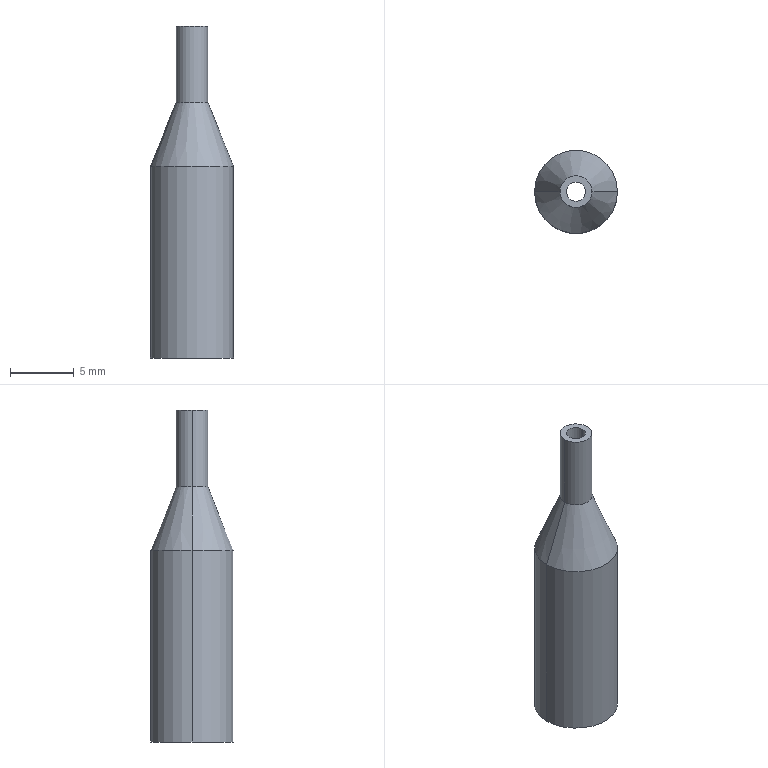Part | SolidWorks | features ICE 2, Chamfer 1, Extrusion 1, HoleWzd 1 | 1 solid | 14 faces | box 6.5 x 6.5 x 26 mm | volume 380.573 mm3 | cylinder 8 | cone 4 | plane 2 | commonest cylinder face diameters 1.5 x2 2.5 x2 4.2 x2 6.5 x2
STEP:
#1=CARTESIAN_POINT('',(-0.75,0.,15.811));
#2=VERTEX_POINT('',#1);
#3=CARTESIAN_POINT('',(0.75,0.,15.811));
#4=VERTEX_POINT('',#3);
#5=CARTESIAN_POINT('',(0.,0.,15.811));
#6=DIRECTION('',(0.,0.,1.));
#7=DIRECTION('',(-1.,0.,0.));
#8=AXIS2_PLACEMENT_3D('',#5,#6,#7);
#9=CIRCLE('',#8,0.75);
#10=EDGE_CURVE('',#2,#4,#9,.T.);
#11=ORIENTED_EDGE('',*,*,#10,.F.);
#12=CARTESIAN_POINT('',(-0.75,0.,26.));
#13=VERTEX_POINT('',#12);
#14=CARTESIAN_POINT('',(-0.75,0.,0.));
#15=DIRECTION('',(0.,0.,1.));
#16=VECTOR('',#15,1000.);
#17=LINE('',#14,#16);
#18=EDGE_CURVE('',#2,#13,#17,.T.);
#19=ORIENTED_EDGE('',*,*,#18,.T.);
#20=CARTESIAN_POINT('',(0.75,0.,26.));
#21=VERTEX_POINT('',#20);
#22=CARTESIAN_POINT('',(0.,0.,26.));
#23=DIRECTION('',(0.,0.,1.));
#24=DIRECTION('',(1.,0.,0.));
#25=AXIS2_PLACEMENT_3D('',#22,#23,#24);
#26=CIRCLE('',#25,0.75);
#27=EDGE_CURVE('',#13,#21,#26,.T.);
#28=ORIENTED_EDGE('',*,*,#27,.T.);
#29=CARTESIAN_POINT('',(0.75,0.,0.));
#30=DIRECTION('',(0.,0.,1.));
#31=VECTOR('',#30,1000.);
#32=LINE('',#29,#31);
#33=EDGE_CURVE('',#4,#21,#32,.T.);
#34=ORIENTED_EDGE('',*,*,#33,.F.);
#35=EDGE_LOOP('',(#11,#19,#28,#34));
#36=FACE_OUTER_BOUND('',#35,.T.);
#37=CARTESIAN_POINT('',(0.,0.,0.));
#38=DIRECTION('',(0.,0.,1.));
#39=DIRECTION('',(1.,0.,0.));
#40=AXIS2_PLACEMENT_3D('',#37,#38,#39);
#41=CYLINDRICAL_SURFACE('',#40,0.75);
#42=ADVANCED_FACE('',(#36),#41,.F.);
#43=CARTESIAN_POINT('',(2.1,0.,15.));
#44=VERTEX_POINT('',#43);
#45=CARTESIAN_POINT('',(-2.1,0.,15.));
#46=VERTEX_POINT('',#45);
#47=CARTESIAN_POINT('',(0.,0.,15.));
#48=DIRECTION('',(0.,0.,-1.));
#49=DIRECTION('',(-1.,0.,0.));
#50=AXIS2_PLACEMENT_3D('',#47,#48,#49);
#51=CIRCLE('',#50,2.1);
#52=EDGE_CURVE('',#44,#46,#51,.T.);
#53=ORIENTED_EDGE('',*,*,#52,.F.);
#54=CARTESIAN_POINT('',(2.1,0.,0.));
#55=VERTEX_POINT('',#54);
#56=CARTESIAN_POINT('',(2.1,0.,0.));
#57=DIRECTION('',(0.,0.,-1.));
#58=VECTOR('',#57,1000.);
#59=LINE('',#56,#58);
#60=EDGE_CURVE('',#44,#55,#59,.T.);
#61=ORIENTED_EDGE('',*,*,#60,.T.);
#62=CARTESIAN_POINT('',(-2.1,0.,0.));
#63=VERTEX_POINT('',#62);
#64=CARTESIAN_POINT('',(0.,0.,0.));
#65=DIRECTION('',(0.,0.,-1.));
#66=DIRECTION('',(-1.,0.,0.));
#67=AXIS2_PLACEMENT_3D('',#64,#65,#66);
#68=CIRCLE('',#67,2.1);
#69=EDGE_CURVE('',#55,#63,#68,.T.);
#70=ORIENTED_EDGE('',*,*,#69,.T.);
#71=CARTESIAN_POINT('',(-2.1,0.,0.));
#72=DIRECTION('',(0.,0.,-1.));
#73=VECTOR('',#72,1000.);
#74=LINE('',#71,#73);
#75=EDGE_CURVE('',#46,#63,#74,.T.);
#76=ORIENTED_EDGE('',*,*,#75,.F.);
#77=EDGE_LOOP('',(#53,#61,#70,#76));
#78=FACE_OUTER_BOUND('',#77,.T.);
#79=CARTESIAN_POINT('',(0.,0.,0.));
#80=DIRECTION('',(0.,0.,-1.));
#81=DIRECTION('',(-1.,0.,0.));
#82=AXIS2_PLACEMENT_3D('',#79,#80,#81);
#83=CYLINDRICAL_SURFACE('',#82,2.1);
#84=ADVANCED_FACE('',(#78),#83,.F.);
#85=ORIENTED_EDGE('',*,*,#10,.T.);
#86=CARTESIAN_POINT('',(2.1,0.,15.));
#87=DIRECTION('',(0.8572,0.,-0.515));
#88=VECTOR('',#87,1000.);
#89=LINE('',#86,#88);
#90=EDGE_CURVE('',#4,#44,#89,.T.);
#91=ORIENTED_EDGE('',*,*,#90,.T.);
#92=ORIENTED_EDGE('',*,*,#52,.T.);
#93=CARTESIAN_POINT('',(-2.1,0.,15.));
#94=DIRECTION('',(-0.8572,0.,-0.515));
#95=VECTOR('',#94,1000.);
#96=LINE('',#93,#95);
#97=EDGE_CURVE('',#2,#46,#96,.T.);
#98=ORIENTED_EDGE('',*,*,#97,.F.);
#99=EDGE_LOOP('',(#85,#91,#92,#98));
#100=FACE_OUTER_BOUND('',#99,.T.);
#101=CARTESIAN_POINT('',(0.,0.,15.));
#102=DIRECTION('',(0.,0.,-1.));
#103=DIRECTION('',(-1.,0.,0.));
#104=AXIS2_PLACEMENT_3D('',#101,#102,#103);
#105=CONICAL_SURFACE('',#104,2.1,1.03);
#106=ADVANCED_FACE('',(#100),#105,.F.);
#107=CARTESIAN_POINT('',(1.25,0.,20.));
#108=VERTEX_POINT('',#107);
#109=CARTESIAN_POINT('',(-1.25,0.,20.));
#110=VERTEX_POINT('',#109);
#111=CARTESIAN_POINT('',(0.,0.,20.));
#112=DIRECTION('',(0.,0.,1.));
#113=DIRECTION('',(1.,0.,0.));
#114=AXIS2_PLACEMENT_3D('',#111,#112,#113);
#115=CIRCLE('',#114,1.25);
#116=EDGE_CURVE('',#108,#110,#115,.T.);
#117=ORIENTED_EDGE('',*,*,#116,.F.);
#118=CARTESIAN_POINT('',(3.25,0.,15.));
#119=VERTEX_POINT('',#118);
#120=CARTESIAN_POINT('',(1.25,0.,20.));
#121=DIRECTION('',(0.3714,0.,-0.9285));
#122=VECTOR('',#121,1000.);
#123=LINE('',#120,#122);
#124=EDGE_CURVE('',#108,#119,#123,.T.);
#125=ORIENTED_EDGE('',*,*,#124,.T.);
#126=CARTESIAN_POINT('',(-3.25,0.,15.));
#127=VERTEX_POINT('',#126);
#128=CARTESIAN_POINT('',(0.,0.,15.));
#129=DIRECTION('',(0.,0.,-1.));
#130=DIRECTION('',(1.,0.,0.));
#131=AXIS2_PLACEMENT_3D('',#128,#129,#130);
#132=CIRCLE('',#131,3.25);
#133=EDGE_CURVE('',#127,#119,#132,.T.);
#134=ORIENTED_EDGE('',*,*,#133,.F.);
#135=CARTESIAN_POINT('',(-1.25,0.,20.));
#136=DIRECTION('',(-0.3714,0.,-0.9285));
#137=VECTOR('',#136,1000.);
#138=LINE('',#135,#137);
#139=EDGE_CURVE('',#110,#127,#138,.T.);
#140=ORIENTED_EDGE('',*,*,#139,.F.);
#141=EDGE_LOOP('',(#117,#125,#134,#140));
#142=FACE_OUTER_BOUND('',#141,.T.);
#143=CARTESIAN_POINT('',(0.,0.,20.));
#144=DIRECTION('',(0.,0.,-1.));
#145=DIRECTION('',(-1.,0.,0.));
#146=AXIS2_PLACEMENT_3D('',#143,#144,#145);
#147=CONICAL_SURFACE('',#146,1.25,0.3805);
#148=ADVANCED_FACE('',(#142),#147,.T.);
#149=CARTESIAN_POINT('',(1.25,0.,26.));
#150=VERTEX_POINT('',#149);
#151=CARTESIAN_POINT('',(-1.25,0.,26.));
#152=VERTEX_POINT('',#151);
#153=CARTESIAN_POINT('',(0.,0.,26.));
#154=DIRECTION('',(0.,0.,1.));
#155=DIRECTION('',(1.,0.,0.));
#156=AXIS2_PLACEMENT_3D('',#153,#154,#155);
#157=CIRCLE('',#156,1.25);
#158=EDGE_CURVE('',#150,#152,#157,.T.);
#159=ORIENTED_EDGE('',*,*,#158,.F.);
#160=CARTESIAN_POINT('',(1.25,0.,26.));
#161=DIRECTION('',(0.,0.,-1.));
#162=VECTOR('',#161,1000.);
#163=LINE('',#160,#162);
#164=EDGE_CURVE('',#150,#108,#163,.T.);
#165=ORIENTED_EDGE('',*,*,#164,.T.);
#166=ORIENTED_EDGE('',*,*,#116,.T.);
#167=CARTESIAN_POINT('',(-1.25,0.,26.));
#168=DIRECTION('',(0.,0.,-1.));
#169=VECTOR('',#168,1000.);
#170=LINE('',#167,#169);
#171=EDGE_CURVE('',#152,#110,#170,.T.);
#172=ORIENTED_EDGE('',*,*,#171,.F.);
#173=EDGE_LOOP('',(#159,#165,#166,#172));
#174=FACE_OUTER_BOUND('',#173,.T.);
#175=CARTESIAN_POINT('',(0.,0.,26.));
#176=DIRECTION('',(0.,0.,-1.));
#177=DIRECTION('',(-1.,0.,0.));
#178=AXIS2_PLACEMENT_3D('',#175,#176,#177);
#179=CYLINDRICAL_SURFACE('',#178,1.25);
#180=ADVANCED_FACE('',(#174),#179,.T.);
#181=ORIENTED_EDGE('',*,*,#133,.T.);
#182=CARTESIAN_POINT('',(3.25,0.,0.));
#183=VERTEX_POINT('',#182);
#184=CARTESIAN_POINT('',(3.25,0.,20.));
#185=DIRECTION('',(0.,0.,-1.));
#186=VECTOR('',#185,1000.);
#187=LINE('',#184,#186);
#188=EDGE_CURVE('',#119,#183,#187,.T.);
#189=ORIENTED_EDGE('',*,*,#188,.T.);
#190=CARTESIAN_POINT('',(-3.25,0.,0.));
#191=VERTEX_POINT('',#190);
#192=CARTESIAN_POINT('',(0.,0.,0.));
#193=DIRECTION('',(0.,0.,1.));
#194=DIRECTION('',(1.,0.,0.));
#195=AXIS2_PLACEMENT_3D('',#192,#193,#194);
#196=CIRCLE('',#195,3.25);
#197=EDGE_CURVE('',#183,#191,#196,.T.);
#198=ORIENTED_EDGE('',*,*,#197,.T.);
#199=CARTESIAN_POINT('',(-3.25,0.,20.));
#200=DIRECTION('',(0.,0.,-1.));
#201=VECTOR('',#200,1000.);
#202=LINE('',#199,#201);
#203=EDGE_CURVE('',#127,#191,#202,.T.);
#204=ORIENTED_EDGE('',*,*,#203,.F.);
#205=EDGE_LOOP('',(#181,#189,#198,#204));
#206=FACE_OUTER_BOUND('',#205,.T.);
#207=CARTESIAN_POINT('',(0.,0.,20.));
#208=DIRECTION('',(0.,0.,-1.));
#209=DIRECTION('',(-1.,0.,0.));
#210=AXIS2_PLACEMENT_3D('',#207,#208,#209);
#211=CYLINDRICAL_SURFACE('',#210,3.25);
#212=ADVANCED_FACE('',(#206),#211,.T.);
#213=ORIENTED_EDGE('',*,*,#188,.F.);
#214=CARTESIAN_POINT('',(0.,0.,15.));
#215=DIRECTION('',(0.,0.,-1.));
#216=DIRECTION('',(1.,0.,0.));
#217=AXIS2_PLACEMENT_3D('',#214,#215,#216);
#218=CIRCLE('',#217,3.25);
#219=EDGE_CURVE('',#119,#127,#218,.T.);
#220=ORIENTED_EDGE('',*,*,#219,.T.);
#221=ORIENTED_EDGE('',*,*,#203,.T.);
#222=CARTESIAN_POINT('',(0.,0.,0.));
#223=DIRECTION('',(0.,0.,1.));
#224=DIRECTION('',(1.,0.,0.));
#225=AXIS2_PLACEMENT_3D('',#222,#223,#224);
#226=CIRCLE('',#225,3.25);
#227=EDGE_CURVE('',#191,#183,#226,.T.);
#228=ORIENTED_EDGE('',*,*,#227,.T.);
#229=EDGE_LOOP('',(#213,#220,#221,#228));
#230=FACE_OUTER_BOUND('',#229,.T.);
#231=CARTESIAN_POINT('',(0.,0.,20.));
#232=DIRECTION('',(0.,0.,-1.));
#233=DIRECTION('',(-1.,0.,0.));
#234=AXIS2_PLACEMENT_3D('',#231,#232,#233);
#235=CYLINDRICAL_SURFACE('',#234,3.25);
#236=ADVANCED_FACE('',(#230),#235,.T.);
#237=CARTESIAN_POINT('',(0.,0.,0.));
#238=DIRECTION('',(0.,0.,-1.));
#239=DIRECTION('',(-1.,0.,0.));
#240=AXIS2_PLACEMENT_3D('',#237,#238,#239);
#241=CIRCLE('',#240,2.1);
#242=EDGE_CURVE('',#63,#55,#241,.T.);
#243=ORIENTED_EDGE('',*,*,#242,.F.);
#244=ORIENTED_EDGE('',*,*,#69,.F.);
#245=EDGE_LOOP('',(#243,#244));
#246=FACE_BOUND('',#245,.T.);
#247=ORIENTED_EDGE('',*,*,#227,.F.);
#248=ORIENTED_EDGE('',*,*,#197,.F.);
#249=EDGE_LOOP('',(#247,#248));
#250=FACE_OUTER_BOUND('',#249,.T.);
#251=CARTESIAN_POINT('',(0.,0.,0.));
#252=DIRECTION('',(0.,0.,1.));
#253=DIRECTION('',(1.,0.,0.));
#254=AXIS2_PLACEMENT_3D('',#251,#252,#253);
#255=PLANE('',#254);
#256=ADVANCED_FACE('',(#246,#250),#255,.F.);
#257=ORIENTED_EDGE('',*,*,#164,.F.);
#258=CARTESIAN_POINT('',(0.,0.,26.));
#259=DIRECTION('',(0.,0.,1.));
#260=DIRECTION('',(1.,0.,0.));
#261=AXIS2_PLACEMENT_3D('',#258,#259,#260);
#262=CIRCLE('',#261,1.25);
#263=EDGE_CURVE('',#152,#150,#262,.T.);
#264=ORIENTED_EDGE('',*,*,#263,.F.);
#265=ORIENTED_EDGE('',*,*,#171,.T.);
#266=CARTESIAN_POINT('',(0.,0.,20.));
#267=DIRECTION('',(0.,0.,1.));
#268=DIRECTION('',(1.,0.,0.));
#269=AXIS2_PLACEMENT_3D('',#266,#267,#268);
#270=CIRCLE('',#269,1.25);
#271=EDGE_CURVE('',#110,#108,#270,.T.);
#272=ORIENTED_EDGE('',*,*,#271,.T.);
#273=EDGE_LOOP('',(#257,#264,#265,#272));
#274=FACE_OUTER_BOUND('',#273,.T.);
#275=CARTESIAN_POINT('',(0.,0.,26.));
#276=DIRECTION('',(0.,0.,-1.));
#277=DIRECTION('',(-1.,0.,0.));
#278=AXIS2_PLACEMENT_3D('',#275,#276,#277);
#279=CYLINDRICAL_SURFACE('',#278,1.25);
#280=ADVANCED_FACE('',(#274),#279,.T.);
#281=CARTESIAN_POINT('',(0.,0.,26.));
#282=DIRECTION('',(0.,0.,1.));
#283=DIRECTION('',(1.,0.,0.));
#284=AXIS2_PLACEMENT_3D('',#281,#282,#283);
#285=CIRCLE('',#284,0.75);
#286=EDGE_CURVE('',#21,#13,#285,.T.);
#287=ORIENTED_EDGE('',*,*,#286,.F.);
#288=ORIENTED_EDGE('',*,*,#27,.F.);
#289=EDGE_LOOP('',(#287,#288));
#290=FACE_BOUND('',#289,.T.);
#291=ORIENTED_EDGE('',*,*,#263,.T.);
#292=ORIENTED_EDGE('',*,*,#158,.T.);
#293=EDGE_LOOP('',(#291,#292));
#294=FACE_OUTER_BOUND('',#293,.T.);
#295=CARTESIAN_POINT('',(0.,0.,26.));
#296=DIRECTION('',(0.,0.,1.));
#297=DIRECTION('',(1.,0.,0.));
#298=AXIS2_PLACEMENT_3D('',#295,#296,#297);
#299=PLANE('',#298);
#300=ADVANCED_FACE('',(#290,#294),#299,.T.);
#301=ORIENTED_EDGE('',*,*,#124,.F.);
#302=ORIENTED_EDGE('',*,*,#271,.F.);
#303=ORIENTED_EDGE('',*,*,#139,.T.);
#304=ORIENTED_EDGE('',*,*,#219,.F.);
#305=EDGE_LOOP('',(#301,#302,#303,#304));
#306=FACE_OUTER_BOUND('',#305,.T.);
#307=CARTESIAN_POINT('',(0.,0.,20.));
#308=DIRECTION('',(0.,0.,-1.));
#309=DIRECTION('',(-1.,0.,0.));
#310=AXIS2_PLACEMENT_3D('',#307,#308,#309);
#311=CONICAL_SURFACE('',#310,1.25,0.3805);
#312=ADVANCED_FACE('',(#306),#311,.T.);
#313=ORIENTED_EDGE('',*,*,#90,.F.);
#314=CARTESIAN_POINT('',(0.,0.,15.811));
#315=DIRECTION('',(0.,0.,1.));
#316=DIRECTION('',(-1.,0.,0.));
#317=AXIS2_PLACEMENT_3D('',#314,#315,#316);
#318=CIRCLE('',#317,0.75);
#319=EDGE_CURVE('',#4,#2,#318,.T.);
#320=ORIENTED_EDGE('',*,*,#319,.T.);
#321=ORIENTED_EDGE('',*,*,#97,.T.);
#322=CARTESIAN_POINT('',(0.,0.,15.));
#323=DIRECTION('',(0.,0.,-1.));
#324=DIRECTION('',(-1.,0.,0.));
#325=AXIS2_PLACEMENT_3D('',#322,#323,#324);
#326=CIRCLE('',#325,2.1);
#327=EDGE_CURVE('',#46,#44,#326,.T.);
#328=ORIENTED_EDGE('',*,*,#327,.T.);
#329=EDGE_LOOP('',(#313,#320,#321,#328));
#330=FACE_OUTER_BOUND('',#329,.T.);
#331=CARTESIAN_POINT('',(0.,0.,15.));
#332=DIRECTION('',(0.,0.,-1.));
#333=DIRECTION('',(-1.,0.,0.));
#334=AXIS2_PLACEMENT_3D('',#331,#332,#333);
#335=CONICAL_SURFACE('',#334,2.1,1.03);
#336=ADVANCED_FACE('',(#330),#335,.F.);
#337=ORIENTED_EDGE('',*,*,#60,.F.);
#338=ORIENTED_EDGE('',*,*,#327,.F.);
#339=ORIENTED_EDGE('',*,*,#75,.T.);
#340=ORIENTED_EDGE('',*,*,#242,.T.);
#341=EDGE_LOOP('',(#337,#338,#339,#340));
#342=FACE_OUTER_BOUND('',#341,.T.);
#343=CARTESIAN_POINT('',(0.,0.,0.));
#344=DIRECTION('',(0.,0.,-1.));
#345=DIRECTION('',(-1.,0.,0.));
#346=AXIS2_PLACEMENT_3D('',#343,#344,#345);
#347=CYLINDRICAL_SURFACE('',#346,2.1);
#348=ADVANCED_FACE('',(#342),#347,.F.);
#349=ORIENTED_EDGE('',*,*,#18,.F.);
#350=ORIENTED_EDGE('',*,*,#319,.F.);
#351=ORIENTED_EDGE('',*,*,#33,.T.);
#352=ORIENTED_EDGE('',*,*,#286,.T.);
#353=EDGE_LOOP('',(#349,#350,#351,#352));
#354=FACE_OUTER_BOUND('',#353,.T.);
#355=CARTESIAN_POINT('',(0.,0.,0.));
#356=DIRECTION('',(0.,0.,1.));
#357=DIRECTION('',(1.,0.,0.));
#358=AXIS2_PLACEMENT_3D('',#355,#356,#357);
#359=CYLINDRICAL_SURFACE('',#358,0.75);
#360=ADVANCED_FACE('',(#354),#359,.F.);
#361=CLOSED_SHELL('',(#42,#84,#106,#148,#180,#212,#236,#256,#280,#300,#312,#336,#348,#360));
#362=MANIFOLD_SOLID_BREP('',#361);
#363=CARTESIAN_POINT('',(0.,0.,0.));
#364=DIRECTION('',(0.,0.,1.));
#365=DIRECTION('',(1.,0.,0.));
#366=AXIS2_PLACEMENT_3D('',#363,#364,#365);
#367=(LENGTH_UNIT()NAMED_UNIT(*)SI_UNIT(.MILLI.,.METRE.));
#368=UNCERTAINTY_MEASURE_WITH_UNIT(LENGTH_MEASURE(0.00001),#367,'','');
#369=(NAMED_UNIT(*)PLANE_ANGLE_UNIT()SI_UNIT($,.RADIAN.));
#370=(NAMED_UNIT(*)SI_UNIT($,.STERADIAN.)SOLID_ANGLE_UNIT());
#371=(GEOMETRIC_REPRESENTATION_CONTEXT(3)GLOBAL_UNCERTAINTY_ASSIGNED_CONTEXT((#368))GLOBAL_UNIT_ASSIGNED_CONTEXT((#367,#369,#370))REPRESENTATION_CONTEXT('',''));
#372=ADVANCED_BREP_SHAPE_REPRESENTATION('',(#362,#366),#371);